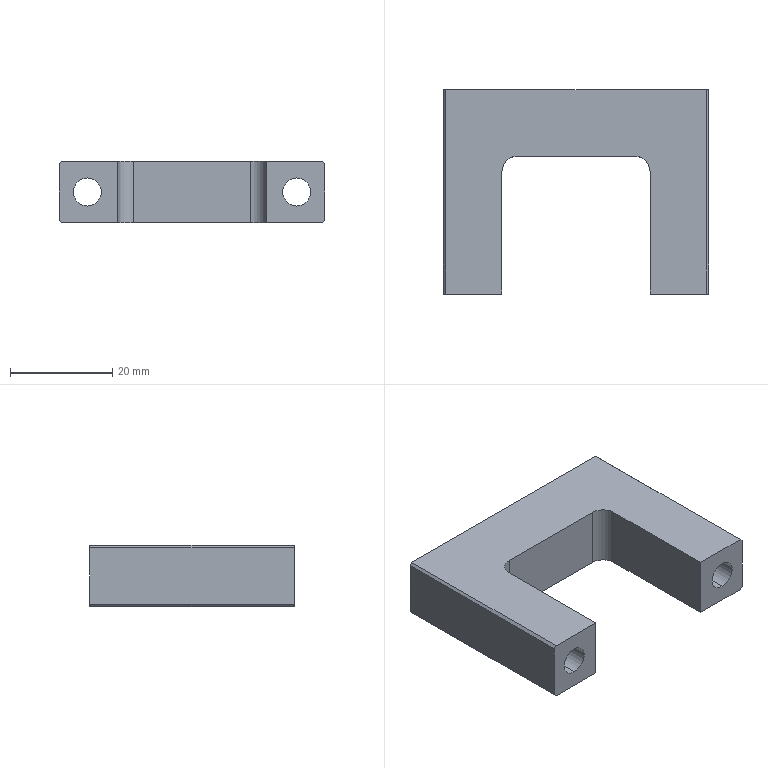Part | SolidWorks | features BaseBody 1 | 1 solid | 26 faces | box 52 x 40 x 12 mm | volume 13065 mm3 | plane 16 | cylinder 10 | commonest cylinder face diameters 5.5 x4 10 x4 6 x2
STEP:
#1=CARTESIAN_POINT('',(-20.5,-5.7,-5.));
#2=VERTEX_POINT('',#1);
#3=CARTESIAN_POINT('',(-20.5,-5.7,5.));
#4=VERTEX_POINT('',#3);
#5=CARTESIAN_POINT('',(-20.5,-5.7,0.));
#6=DIRECTION('',(0.,1.,0.));
#7=DIRECTION('',(0.,0.,1.));
#8=AXIS2_PLACEMENT_3D('',#5,#6,#7);
#9=CIRCLE('',#8,5.);
#10=EDGE_CURVE('',#2,#4,#9,.T.);
#11=ORIENTED_EDGE('',*,*,#10,.F.);
#12=CARTESIAN_POINT('',(-20.5,0.,-5.));
#13=VERTEX_POINT('',#12);
#14=CARTESIAN_POINT('',(-20.5,0.,-5.));
#15=DIRECTION('',(0.,1.,0.));
#16=VECTOR('',#15,1000.);
#17=LINE('',#14,#16);
#18=EDGE_CURVE('',#2,#13,#17,.T.);
#19=ORIENTED_EDGE('',*,*,#18,.T.);
#20=CARTESIAN_POINT('',(-20.5,0.,5.));
#21=VERTEX_POINT('',#20);
#22=CARTESIAN_POINT('',(-20.5,0.,0.));
#23=DIRECTION('',(0.,1.,0.));
#24=DIRECTION('',(0.,0.,1.));
#25=AXIS2_PLACEMENT_3D('',#22,#23,#24);
#26=CIRCLE('',#25,5.);
#27=EDGE_CURVE('',#13,#21,#26,.T.);
#28=ORIENTED_EDGE('',*,*,#27,.T.);
#29=CARTESIAN_POINT('',(-20.5,0.,5.));
#30=DIRECTION('',(0.,1.,0.));
#31=VECTOR('',#30,1000.);
#32=LINE('',#29,#31);
#33=EDGE_CURVE('',#4,#21,#32,.T.);
#34=ORIENTED_EDGE('',*,*,#33,.F.);
#35=EDGE_LOOP('',(#11,#19,#28,#34));
#36=FACE_OUTER_BOUND('',#35,.T.);
#37=CARTESIAN_POINT('',(-20.5,0.,0.));
#38=DIRECTION('',(0.,1.,0.));
#39=DIRECTION('',(0.,0.,1.));
#40=AXIS2_PLACEMENT_3D('',#37,#38,#39);
#41=CYLINDRICAL_SURFACE('',#40,5.);
#42=ADVANCED_FACE('',(#36),#41,.F.);
#43=CARTESIAN_POINT('',(-20.5,-40.,-2.75));
#44=VERTEX_POINT('',#43);
#45=CARTESIAN_POINT('',(-20.5,-40.,2.75));
#46=VERTEX_POINT('',#45);
#47=CARTESIAN_POINT('',(-20.5,-40.,0.));
#48=DIRECTION('',(0.,1.,0.));
#49=DIRECTION('',(-1.,0.,0.));
#50=AXIS2_PLACEMENT_3D('',#47,#48,#49);
#51=CIRCLE('',#50,2.75);
#52=EDGE_CURVE('',#44,#46,#51,.T.);
#53=ORIENTED_EDGE('',*,*,#52,.F.);
#54=CARTESIAN_POINT('',(-20.5,-5.7,-2.75));
#55=VERTEX_POINT('',#54);
#56=CARTESIAN_POINT('',(-20.5,0.,-2.75));
#57=DIRECTION('',(0.,1.,0.));
#58=VECTOR('',#57,1000.);
#59=LINE('',#56,#58);
#60=EDGE_CURVE('',#44,#55,#59,.T.);
#61=ORIENTED_EDGE('',*,*,#60,.T.);
#62=CARTESIAN_POINT('',(-20.5,-5.7,2.75));
#63=VERTEX_POINT('',#62);
#64=CARTESIAN_POINT('',(-20.5,-5.7,0.));
#65=DIRECTION('',(0.,1.,0.));
#66=DIRECTION('',(0.,0.,1.));
#67=AXIS2_PLACEMENT_3D('',#64,#65,#66);
#68=CIRCLE('',#67,2.75);
#69=EDGE_CURVE('',#55,#63,#68,.T.);
#70=ORIENTED_EDGE('',*,*,#69,.T.);
#71=CARTESIAN_POINT('',(-20.5,0.,2.75));
#72=DIRECTION('',(0.,1.,0.));
#73=VECTOR('',#72,1000.);
#74=LINE('',#71,#73);
#75=EDGE_CURVE('',#46,#63,#74,.T.);
#76=ORIENTED_EDGE('',*,*,#75,.F.);
#77=EDGE_LOOP('',(#53,#61,#70,#76));
#78=FACE_OUTER_BOUND('',#77,.T.);
#79=CARTESIAN_POINT('',(-20.5,0.,0.));
#80=DIRECTION('',(0.,1.,0.));
#81=DIRECTION('',(0.,0.,1.));
#82=AXIS2_PLACEMENT_3D('',#79,#80,#81);
#83=CYLINDRICAL_SURFACE('',#82,2.75);
#84=ADVANCED_FACE('',(#78),#83,.F.);
#85=CARTESIAN_POINT('',(20.5,-5.7,-5.));
#86=VERTEX_POINT('',#85);
#87=CARTESIAN_POINT('',(20.5,-5.7,5.));
#88=VERTEX_POINT('',#87);
#89=CARTESIAN_POINT('',(20.5,-5.7,0.));
#90=DIRECTION('',(0.,1.,0.));
#91=DIRECTION('',(0.,0.,1.));
#92=AXIS2_PLACEMENT_3D('',#89,#90,#91);
#93=CIRCLE('',#92,5.);
#94=EDGE_CURVE('',#86,#88,#93,.T.);
#95=ORIENTED_EDGE('',*,*,#94,.F.);
#96=CARTESIAN_POINT('',(20.5,0.,-5.));
#97=VERTEX_POINT('',#96);
#98=CARTESIAN_POINT('',(20.5,0.,-5.));
#99=DIRECTION('',(0.,1.,0.));
#100=VECTOR('',#99,1000.);
#101=LINE('',#98,#100);
#102=EDGE_CURVE('',#86,#97,#101,.T.);
#103=ORIENTED_EDGE('',*,*,#102,.T.);
#104=CARTESIAN_POINT('',(20.5,0.,5.));
#105=VERTEX_POINT('',#104);
#106=CARTESIAN_POINT('',(20.5,0.,0.));
#107=DIRECTION('',(0.,1.,0.));
#108=DIRECTION('',(0.,0.,1.));
#109=AXIS2_PLACEMENT_3D('',#106,#107,#108);
#110=CIRCLE('',#109,5.);
#111=EDGE_CURVE('',#97,#105,#110,.T.);
#112=ORIENTED_EDGE('',*,*,#111,.T.);
#113=CARTESIAN_POINT('',(20.5,0.,5.));
#114=DIRECTION('',(0.,1.,0.));
#115=VECTOR('',#114,1000.);
#116=LINE('',#113,#115);
#117=EDGE_CURVE('',#88,#105,#116,.T.);
#118=ORIENTED_EDGE('',*,*,#117,.F.);
#119=EDGE_LOOP('',(#95,#103,#112,#118));
#120=FACE_OUTER_BOUND('',#119,.T.);
#121=CARTESIAN_POINT('',(20.5,0.,0.));
#122=DIRECTION('',(0.,1.,0.));
#123=DIRECTION('',(0.,0.,1.));
#124=AXIS2_PLACEMENT_3D('',#121,#122,#123);
#125=CYLINDRICAL_SURFACE('',#124,5.);
#126=ADVANCED_FACE('',(#120),#125,.F.);
#127=CARTESIAN_POINT('',(20.5,-40.,-2.75));
#128=VERTEX_POINT('',#127);
#129=CARTESIAN_POINT('',(20.5,-40.,2.75));
#130=VERTEX_POINT('',#129);
#131=CARTESIAN_POINT('',(20.5,-40.,0.));
#132=DIRECTION('',(0.,1.,0.));
#133=DIRECTION('',(-1.,0.,0.));
#134=AXIS2_PLACEMENT_3D('',#131,#132,#133);
#135=CIRCLE('',#134,2.75);
#136=EDGE_CURVE('',#128,#130,#135,.T.);
#137=ORIENTED_EDGE('',*,*,#136,.F.);
#138=CARTESIAN_POINT('',(20.5,-5.7,-2.75));
#139=VERTEX_POINT('',#138);
#140=CARTESIAN_POINT('',(20.5,0.,-2.75));
#141=DIRECTION('',(0.,1.,0.));
#142=VECTOR('',#141,1000.);
#143=LINE('',#140,#142);
#144=EDGE_CURVE('',#128,#139,#143,.T.);
#145=ORIENTED_EDGE('',*,*,#144,.T.);
#146=CARTESIAN_POINT('',(20.5,-5.7,2.75));
#147=VERTEX_POINT('',#146);
#148=CARTESIAN_POINT('',(20.5,-5.7,0.));
#149=DIRECTION('',(0.,1.,0.));
#150=DIRECTION('',(0.,0.,1.));
#151=AXIS2_PLACEMENT_3D('',#148,#149,#150);
#152=CIRCLE('',#151,2.75);
#153=EDGE_CURVE('',#139,#147,#152,.T.);
#154=ORIENTED_EDGE('',*,*,#153,.T.);
#155=CARTESIAN_POINT('',(20.5,0.,2.75));
#156=DIRECTION('',(0.,1.,0.));
#157=VECTOR('',#156,1000.);
#158=LINE('',#155,#157);
#159=EDGE_CURVE('',#130,#147,#158,.T.);
#160=ORIENTED_EDGE('',*,*,#159,.F.);
#161=EDGE_LOOP('',(#137,#145,#154,#160));
#162=FACE_OUTER_BOUND('',#161,.T.);
#163=CARTESIAN_POINT('',(20.5,0.,0.));
#164=DIRECTION('',(0.,1.,0.));
#165=DIRECTION('',(0.,0.,1.));
#166=AXIS2_PLACEMENT_3D('',#163,#164,#165);
#167=CYLINDRICAL_SURFACE('',#166,2.75);
#168=ADVANCED_FACE('',(#162),#167,.F.);
#169=CARTESIAN_POINT('',(-14.5,-16.,6.));
#170=VERTEX_POINT('',#169);
#171=CARTESIAN_POINT('',(-11.5,-13.,6.));
#172=VERTEX_POINT('',#171);
#173=CARTESIAN_POINT('',(-11.5,-16.,6.));
#174=DIRECTION('',(0.,0.,-1.));
#175=DIRECTION('',(-1.,0.,0.));
#176=AXIS2_PLACEMENT_3D('',#173,#174,#175);
#177=CIRCLE('',#176,3.);
#178=EDGE_CURVE('',#170,#172,#177,.T.);
#179=ORIENTED_EDGE('',*,*,#178,.F.);
#180=CARTESIAN_POINT('',(-14.5,-16.,-6.));
#181=VERTEX_POINT('',#180);
#182=CARTESIAN_POINT('',(-14.5,-16.,6.));
#183=DIRECTION('',(0.,0.,1.));
#184=VECTOR('',#183,1000.);
#185=LINE('',#182,#184);
#186=EDGE_CURVE('',#181,#170,#185,.T.);
#187=ORIENTED_EDGE('',*,*,#186,.F.);
#188=CARTESIAN_POINT('',(-11.5,-13.,-6.));
#189=VERTEX_POINT('',#188);
#190=CARTESIAN_POINT('',(-11.5,-16.,-6.));
#191=DIRECTION('',(0.,0.,1.));
#192=DIRECTION('',(-1.,0.,0.));
#193=AXIS2_PLACEMENT_3D('',#190,#191,#192);
#194=CIRCLE('',#193,3.);
#195=EDGE_CURVE('',#189,#181,#194,.T.);
#196=ORIENTED_EDGE('',*,*,#195,.F.);
#197=CARTESIAN_POINT('',(-11.5,-13.,-6.));
#198=DIRECTION('',(0.,0.,-1.));
#199=VECTOR('',#198,1000.);
#200=LINE('',#197,#199);
#201=EDGE_CURVE('',#172,#189,#200,.T.);
#202=ORIENTED_EDGE('',*,*,#201,.F.);
#203=EDGE_LOOP('',(#179,#187,#196,#202));
#204=FACE_OUTER_BOUND('',#203,.T.);
#205=CARTESIAN_POINT('',(-11.5,-16.,6.));
#206=DIRECTION('',(0.,0.,1.));
#207=DIRECTION('',(1.,0.,0.));
#208=AXIS2_PLACEMENT_3D('',#205,#206,#207);
#209=CYLINDRICAL_SURFACE('',#208,3.);
#210=ADVANCED_FACE('',(#204),#209,.F.);
#211=CARTESIAN_POINT('',(11.5,-13.,6.));
#212=VERTEX_POINT('',#211);
#213=CARTESIAN_POINT('',(14.5,-16.,6.));
#214=VERTEX_POINT('',#213);
#215=CARTESIAN_POINT('',(11.5,-16.,6.));
#216=DIRECTION('',(0.,0.,-1.));
#217=DIRECTION('',(-1.,0.,0.));
#218=AXIS2_PLACEMENT_3D('',#215,#216,#217);
#219=CIRCLE('',#218,3.);
#220=EDGE_CURVE('',#212,#214,#219,.T.);
#221=ORIENTED_EDGE('',*,*,#220,.F.);
#222=CARTESIAN_POINT('',(11.5,-13.,-6.));
#223=VERTEX_POINT('',#222);
#224=CARTESIAN_POINT('',(11.5,-13.,6.));
#225=DIRECTION('',(0.,0.,1.));
#226=VECTOR('',#225,1000.);
#227=LINE('',#224,#226);
#228=EDGE_CURVE('',#223,#212,#227,.T.);
#229=ORIENTED_EDGE('',*,*,#228,.F.);
#230=CARTESIAN_POINT('',(14.5,-16.,-6.));
#231=VERTEX_POINT('',#230);
#232=CARTESIAN_POINT('',(11.5,-16.,-6.));
#233=DIRECTION('',(0.,0.,1.));
#234=DIRECTION('',(-1.,0.,0.));
#235=AXIS2_PLACEMENT_3D('',#232,#233,#234);
#236=CIRCLE('',#235,3.);
#237=EDGE_CURVE('',#231,#223,#236,.T.);
#238=ORIENTED_EDGE('',*,*,#237,.F.);
#239=CARTESIAN_POINT('',(14.5,-16.,-6.));
#240=DIRECTION('',(0.,0.,-1.));
#241=VECTOR('',#240,1000.);
#242=LINE('',#239,#241);
#243=EDGE_CURVE('',#214,#231,#242,.T.);
#244=ORIENTED_EDGE('',*,*,#243,.F.);
#245=EDGE_LOOP('',(#221,#229,#238,#244));
#246=FACE_OUTER_BOUND('',#245,.T.);
#247=CARTESIAN_POINT('',(11.5,-16.,6.));
#248=DIRECTION('',(0.,0.,1.));
#249=DIRECTION('',(1.,0.,0.));
#250=AXIS2_PLACEMENT_3D('',#247,#248,#249);
#251=CYLINDRICAL_SURFACE('',#250,3.);
#252=ADVANCED_FACE('',(#246),#251,.F.);
#253=CARTESIAN_POINT('',(-26.,0.,5.5));
#254=VERTEX_POINT('',#253);
#255=CARTESIAN_POINT('',(-25.5,0.,6.));
#256=VERTEX_POINT('',#255);
#257=CARTESIAN_POINT('',(-25.5,0.,6.));
#258=DIRECTION('',(0.7071,0.,0.7071));
#259=VECTOR('',#258,1000.);
#260=LINE('',#257,#259);
#261=EDGE_CURVE('',#254,#256,#260,.T.);
#262=ORIENTED_EDGE('',*,*,#261,.F.);
#263=CARTESIAN_POINT('',(-26.,-40.,5.5));
#264=VERTEX_POINT('',#263);
#265=CARTESIAN_POINT('',(-26.,-40.,5.5));
#266=DIRECTION('',(0.,1.,0.));
#267=VECTOR('',#266,1000.);
#268=LINE('',#265,#267);
#269=EDGE_CURVE('',#264,#254,#268,.T.);
#270=ORIENTED_EDGE('',*,*,#269,.F.);
#271=CARTESIAN_POINT('',(-25.5,-40.,6.));
#272=VERTEX_POINT('',#271);
#273=CARTESIAN_POINT('',(-25.5,-40.,6.));
#274=DIRECTION('',(-0.7071,0.,-0.7071));
#275=VECTOR('',#274,1000.);
#276=LINE('',#273,#275);
#277=EDGE_CURVE('',#272,#264,#276,.T.);
#278=ORIENTED_EDGE('',*,*,#277,.F.);
#279=CARTESIAN_POINT('',(-25.5,0.,6.));
#280=DIRECTION('',(0.,-1.,0.));
#281=VECTOR('',#280,1000.);
#282=LINE('',#279,#281);
#283=EDGE_CURVE('',#256,#272,#282,.T.);
#284=ORIENTED_EDGE('',*,*,#283,.F.);
#285=EDGE_LOOP('',(#262,#270,#278,#284));
#286=FACE_OUTER_BOUND('',#285,.T.);
#287=CARTESIAN_POINT('',(-25.5,0.,6.));
#288=DIRECTION('',(0.7071,0.,-0.7071));
#289=DIRECTION('',(0.,-1.,0.));
#290=AXIS2_PLACEMENT_3D('',#287,#288,#289);
#291=PLANE('',#290);
#292=ADVANCED_FACE('',(#286),#291,.F.);
#293=CARTESIAN_POINT('',(-25.5,0.,-6.));
#294=VERTEX_POINT('',#293);
#295=CARTESIAN_POINT('',(-26.,0.,-5.5));
#296=VERTEX_POINT('',#295);
#297=CARTESIAN_POINT('',(-26.,0.,-5.5));
#298=DIRECTION('',(-0.7071,0.,0.7071));
#299=VECTOR('',#298,1000.);
#300=LINE('',#297,#299);
#301=EDGE_CURVE('',#294,#296,#300,.T.);
#302=ORIENTED_EDGE('',*,*,#301,.F.);
#303=CARTESIAN_POINT('',(-25.5,-40.,-6.));
#304=VERTEX_POINT('',#303);
#305=CARTESIAN_POINT('',(-25.5,0.,-6.));
#306=DIRECTION('',(0.,1.,0.));
#307=VECTOR('',#306,1000.);
#308=LINE('',#305,#307);
#309=EDGE_CURVE('',#304,#294,#308,.T.);
#310=ORIENTED_EDGE('',*,*,#309,.F.);
#311=CARTESIAN_POINT('',(-26.,-40.,-5.5));
#312=VERTEX_POINT('',#311);
#313=CARTESIAN_POINT('',(-26.,-40.,-5.5));
#314=DIRECTION('',(0.7071,0.,-0.7071));
#315=VECTOR('',#314,1000.);
#316=LINE('',#313,#315);
#317=EDGE_CURVE('',#312,#304,#316,.T.);
#318=ORIENTED_EDGE('',*,*,#317,.F.);
#319=CARTESIAN_POINT('',(-26.,-40.,-5.5));
#320=DIRECTION('',(0.,-1.,0.));
#321=VECTOR('',#320,1000.);
#322=LINE('',#319,#321);
#323=EDGE_CURVE('',#296,#312,#322,.T.);
#324=ORIENTED_EDGE('',*,*,#323,.F.);
#325=EDGE_LOOP('',(#302,#310,#318,#324));
#326=FACE_OUTER_BOUND('',#325,.T.);
#327=CARTESIAN_POINT('',(-26.,-40.,-5.5));
#328=DIRECTION('',(-0.7071,0.,-0.7071));
#329=DIRECTION('',(-0.7071,0.,0.7071));
#330=AXIS2_PLACEMENT_3D('',#327,#328,#329);
#331=PLANE('',#330);
#332=ADVANCED_FACE('',(#326),#331,.T.);
#333=CARTESIAN_POINT('',(26.,-40.,5.5));
#334=VERTEX_POINT('',#333);
#335=CARTESIAN_POINT('',(25.5,-40.,6.));
#336=VERTEX_POINT('',#335);
#337=CARTESIAN_POINT('',(25.5,-40.,6.));
#338=DIRECTION('',(-0.7071,0.,0.7071));
#339=VECTOR('',#338,1000.);
#340=LINE('',#337,#339);
#341=EDGE_CURVE('',#334,#336,#340,.T.);
#342=ORIENTED_EDGE('',*,*,#341,.F.);
#343=CARTESIAN_POINT('',(26.,0.,5.5));
#344=VERTEX_POINT('',#343);
#345=CARTESIAN_POINT('',(26.,0.,5.5));
#346=DIRECTION('',(0.,-1.,0.));
#347=VECTOR('',#346,1000.);
#348=LINE('',#345,#347);
#349=EDGE_CURVE('',#344,#334,#348,.T.);
#350=ORIENTED_EDGE('',*,*,#349,.F.);
#351=CARTESIAN_POINT('',(25.5,0.,6.));
#352=VERTEX_POINT('',#351);
#353=CARTESIAN_POINT('',(25.5,0.,6.));
#354=DIRECTION('',(0.7071,0.,-0.7071));
#355=VECTOR('',#354,1000.);
#356=LINE('',#353,#355);
#357=EDGE_CURVE('',#352,#344,#356,.T.);
#358=ORIENTED_EDGE('',*,*,#357,.F.);
#359=CARTESIAN_POINT('',(25.5,0.,6.));
#360=DIRECTION('',(0.,1.,0.));
#361=VECTOR('',#360,1000.);
#362=LINE('',#359,#361);
#363=EDGE_CURVE('',#336,#352,#362,.T.);
#364=ORIENTED_EDGE('',*,*,#363,.F.);
#365=EDGE_LOOP('',(#342,#350,#358,#364));
#366=FACE_OUTER_BOUND('',#365,.T.);
#367=CARTESIAN_POINT('',(25.5,0.,6.));
#368=DIRECTION('',(-0.7071,0.,-0.7071));
#369=DIRECTION('',(-0.7071,0.,0.7071));
#370=AXIS2_PLACEMENT_3D('',#367,#368,#369);
#371=PLANE('',#370);
#372=ADVANCED_FACE('',(#366),#371,.F.);
#373=CARTESIAN_POINT('',(25.5,-40.,-6.));
#374=VERTEX_POINT('',#373);
#375=CARTESIAN_POINT('',(26.,-40.,-5.5));
#376=VERTEX_POINT('',#375);
#377=CARTESIAN_POINT('',(26.,-40.,-5.5));
#378=DIRECTION('',(0.7071,0.,0.7071));
#379=VECTOR('',#378,1000.);
#380=LINE('',#377,#379);
#381=EDGE_CURVE('',#374,#376,#380,.T.);
#382=ORIENTED_EDGE('',*,*,#381,.F.);
#383=CARTESIAN_POINT('',(25.5,0.,-6.));
#384=VERTEX_POINT('',#383);
#385=CARTESIAN_POINT('',(25.5,-40.,-6.));
#386=DIRECTION('',(0.,-1.,0.));
#387=VECTOR('',#386,1000.);
#388=LINE('',#385,#387);
#389=EDGE_CURVE('',#384,#374,#388,.T.);
#390=ORIENTED_EDGE('',*,*,#389,.F.);
#391=CARTESIAN_POINT('',(26.,0.,-5.5));
#392=VERTEX_POINT('',#391);
#393=CARTESIAN_POINT('',(26.,0.,-5.5));
#394=DIRECTION('',(-0.7071,0.,-0.7071));
#395=VECTOR('',#394,1000.);
#396=LINE('',#393,#395);
#397=EDGE_CURVE('',#392,#384,#396,.T.);
#398=ORIENTED_EDGE('',*,*,#397,.F.);
#399=CARTESIAN_POINT('',(26.,0.,-5.5));
#400=DIRECTION('',(0.,1.,0.));
#401=VECTOR('',#400,1000.);
#402=LINE('',#399,#401);
#403=EDGE_CURVE('',#376,#392,#402,.T.);
#404=ORIENTED_EDGE('',*,*,#403,.F.);
#405=EDGE_LOOP('',(#382,#390,#398,#404));
#406=FACE_OUTER_BOUND('',#405,.T.);
#407=CARTESIAN_POINT('',(26.,0.,-5.5));
#408=DIRECTION('',(0.7071,0.,-0.7071));
#409=DIRECTION('',(0.,-1.,0.));
#410=AXIS2_PLACEMENT_3D('',#407,#408,#409);
#411=PLANE('',#410);
#412=ADVANCED_FACE('',(#406),#411,.T.);
#413=CARTESIAN_POINT('',(-20.5,-5.7,0.));
#414=DIRECTION('',(0.,1.,0.));
#415=DIRECTION('',(0.,0.,1.));
#416=AXIS2_PLACEMENT_3D('',#413,#414,#415);
#417=CIRCLE('',#416,2.75);
#418=EDGE_CURVE('',#63,#55,#417,.T.);
#419=ORIENTED_EDGE('',*,*,#418,.F.);
#420=ORIENTED_EDGE('',*,*,#69,.F.);
#421=EDGE_LOOP('',(#419,#420));
#422=FACE_BOUND('',#421,.T.);
#423=CARTESIAN_POINT('',(-20.5,-5.7,0.));
#424=DIRECTION('',(0.,1.,0.));
#425=DIRECTION('',(0.,0.,1.));
#426=AXIS2_PLACEMENT_3D('',#423,#424,#425);
#427=CIRCLE('',#426,5.);
#428=EDGE_CURVE('',#4,#2,#427,.T.);
#429=ORIENTED_EDGE('',*,*,#428,.T.);
#430=ORIENTED_EDGE('',*,*,#10,.T.);
#431=EDGE_LOOP('',(#429,#430));
#432=FACE_OUTER_BOUND('',#431,.T.);
#433=CARTESIAN_POINT('',(-17.75,-5.7,0.));
#434=DIRECTION('',(0.,-1.,0.));
#435=DIRECTION('',(0.,0.,-1.));
#436=AXIS2_PLACEMENT_3D('',#433,#434,#435);
#437=PLANE('',#436);
#438=ADVANCED_FACE('',(#422,#432),#437,.F.);
#439=CARTESIAN_POINT('',(20.5,-5.7,0.));
#440=DIRECTION('',(0.,1.,0.));
#441=DIRECTION('',(0.,0.,1.));
#442=AXIS2_PLACEMENT_3D('',#439,#440,#441);
#443=CIRCLE('',#442,2.75);
#444=EDGE_CURVE('',#147,#139,#443,.T.);
#445=ORIENTED_EDGE('',*,*,#444,.F.);
#446=ORIENTED_EDGE('',*,*,#153,.F.);
#447=EDGE_LOOP('',(#445,#446));
#448=FACE_BOUND('',#447,.T.);
#449=CARTESIAN_POINT('',(20.5,-5.7,0.));
#450=DIRECTION('',(0.,1.,0.));
#451=DIRECTION('',(0.,0.,1.));
#452=AXIS2_PLACEMENT_3D('',#449,#450,#451);
#453=CIRCLE('',#452,5.);
#454=EDGE_CURVE('',#88,#86,#453,.T.);
#455=ORIENTED_EDGE('',*,*,#454,.T.);
#456=ORIENTED_EDGE('',*,*,#94,.T.);
#457=EDGE_LOOP('',(#455,#456));
#458=FACE_OUTER_BOUND('',#457,.T.);
#459=CARTESIAN_POINT('',(23.25,-5.7,0.));
#460=DIRECTION('',(0.,-1.,0.));
#461=DIRECTION('',(0.,0.,-1.));
#462=AXIS2_PLACEMENT_3D('',#459,#460,#461);
#463=PLANE('',#462);
#464=ADVANCED_FACE('',(#448,#458),#463,.F.);
#465=CARTESIAN_POINT('',(-26.,0.,-6.));
#466=DIRECTION('',(-1.,0.,0.));
#467=VECTOR('',#466,1000.);
#468=LINE('',#465,#467);
#469=EDGE_CURVE('',#384,#294,#468,.T.);
#470=ORIENTED_EDGE('',*,*,#469,.F.);
#471=ORIENTED_EDGE('',*,*,#389,.T.);
#472=CARTESIAN_POINT('',(14.5,-40.,-6.));
#473=VERTEX_POINT('',#472);
#474=CARTESIAN_POINT('',(26.,-40.,-6.));
#475=DIRECTION('',(1.,0.,0.));
#476=VECTOR('',#475,1000.);
#477=LINE('',#474,#476);
#478=EDGE_CURVE('',#473,#374,#477,.T.);
#479=ORIENTED_EDGE('',*,*,#478,.F.);
#480=CARTESIAN_POINT('',(14.5,-40.,-6.));
#481=DIRECTION('',(0.,-1.,0.));
#482=VECTOR('',#481,1000.);
#483=LINE('',#480,#482);
#484=EDGE_CURVE('',#231,#473,#483,.T.);
#485=ORIENTED_EDGE('',*,*,#484,.F.);
#486=ORIENTED_EDGE('',*,*,#237,.T.);
#487=CARTESIAN_POINT('',(14.5,-13.,-6.));
#488=DIRECTION('',(1.,0.,0.));
#489=VECTOR('',#488,1000.);
#490=LINE('',#487,#489);
#491=EDGE_CURVE('',#189,#223,#490,.T.);
#492=ORIENTED_EDGE('',*,*,#491,.F.);
#493=ORIENTED_EDGE('',*,*,#195,.T.);
#494=CARTESIAN_POINT('',(-14.5,-40.,-6.));
#495=VERTEX_POINT('',#494);
#496=CARTESIAN_POINT('',(-14.5,-13.,-6.));
#497=DIRECTION('',(0.,1.,0.));
#498=VECTOR('',#497,1000.);
#499=LINE('',#496,#498);
#500=EDGE_CURVE('',#495,#181,#499,.T.);
#501=ORIENTED_EDGE('',*,*,#500,.F.);
#502=CARTESIAN_POINT('',(-14.5,-40.,-6.));
#503=DIRECTION('',(1.,0.,0.));
#504=VECTOR('',#503,1000.);
#505=LINE('',#502,#504);
#506=EDGE_CURVE('',#304,#495,#505,.T.);
#507=ORIENTED_EDGE('',*,*,#506,.F.);
#508=ORIENTED_EDGE('',*,*,#309,.T.);
#509=EDGE_LOOP('',(#470,#471,#479,#485,#486,#492,#493,#501,#507,#508));
#510=FACE_OUTER_BOUND('',#509,.T.);
#511=CARTESIAN_POINT('',(0.,0.,-6.));
#512=DIRECTION('',(0.,0.,-1.));
#513=DIRECTION('',(0.,-1.,0.));
#514=AXIS2_PLACEMENT_3D('',#511,#512,#513);
#515=PLANE('',#514);
#516=ADVANCED_FACE('',(#510),#515,.T.);
#517=CARTESIAN_POINT('',(14.5,-40.,6.));
#518=VERTEX_POINT('',#517);
#519=CARTESIAN_POINT('',(26.,-40.,6.));
#520=DIRECTION('',(1.,0.,0.));
#521=VECTOR('',#520,1000.);
#522=LINE('',#519,#521);
#523=EDGE_CURVE('',#518,#336,#522,.T.);
#524=ORIENTED_EDGE('',*,*,#523,.T.);
#525=ORIENTED_EDGE('',*,*,#363,.T.);
#526=CARTESIAN_POINT('',(-26.,0.,6.));
#527=DIRECTION('',(-1.,0.,0.));
#528=VECTOR('',#527,1000.);
#529=LINE('',#526,#528);
#530=EDGE_CURVE('',#352,#256,#529,.T.);
#531=ORIENTED_EDGE('',*,*,#530,.T.);
#532=ORIENTED_EDGE('',*,*,#283,.T.);
#533=CARTESIAN_POINT('',(-14.5,-40.,6.));
#534=VERTEX_POINT('',#533);
#535=CARTESIAN_POINT('',(-14.5,-40.,6.));
#536=DIRECTION('',(1.,0.,0.));
#537=VECTOR('',#536,1000.);
#538=LINE('',#535,#537);
#539=EDGE_CURVE('',#272,#534,#538,.T.);
#540=ORIENTED_EDGE('',*,*,#539,.T.);
#541=CARTESIAN_POINT('',(-14.5,-13.,6.));
#542=DIRECTION('',(0.,1.,0.));
#543=VECTOR('',#542,1000.);
#544=LINE('',#541,#543);
#545=EDGE_CURVE('',#534,#170,#544,.T.);
#546=ORIENTED_EDGE('',*,*,#545,.T.);
#547=ORIENTED_EDGE('',*,*,#178,.T.);
#548=CARTESIAN_POINT('',(14.5,-13.,6.));
#549=DIRECTION('',(1.,0.,0.));
#550=VECTOR('',#549,1000.);
#551=LINE('',#548,#550);
#552=EDGE_CURVE('',#172,#212,#551,.T.);
#553=ORIENTED_EDGE('',*,*,#552,.T.);
#554=ORIENTED_EDGE('',*,*,#220,.T.);
#555=CARTESIAN_POINT('',(14.5,-40.,6.));
#556=DIRECTION('',(0.,-1.,0.));
#557=VECTOR('',#556,1000.);
#558=LINE('',#555,#557);
#559=EDGE_CURVE('',#214,#518,#558,.T.);
#560=ORIENTED_EDGE('',*,*,#559,.T.);
#561=EDGE_LOOP('',(#524,#525,#531,#532,#540,#546,#547,#553,#554,#560));
#562=FACE_OUTER_BOUND('',#561,.T.);
#563=CARTESIAN_POINT('',(0.,0.,6.));
#564=DIRECTION('',(0.,0.,-1.));
#565=DIRECTION('',(0.,-1.,0.));
#566=AXIS2_PLACEMENT_3D('',#563,#564,#565);
#567=PLANE('',#566);
#568=ADVANCED_FACE('',(#562),#567,.F.);
#569=CARTESIAN_POINT('',(-26.,0.,6.));
#570=DIRECTION('',(0.,0.,-1.));
#571=VECTOR('',#570,1000.);
#572=LINE('',#569,#571);
#573=EDGE_CURVE('',#254,#296,#572,.T.);
#574=ORIENTED_EDGE('',*,*,#573,.T.);
#575=ORIENTED_EDGE('',*,*,#323,.T.);
#576=CARTESIAN_POINT('',(-26.,-40.,6.));
#577=DIRECTION('',(0.,0.,-1.));
#578=VECTOR('',#577,1000.);
#579=LINE('',#576,#578);
#580=EDGE_CURVE('',#264,#312,#579,.T.);
#581=ORIENTED_EDGE('',*,*,#580,.F.);
#582=ORIENTED_EDGE('',*,*,#269,.T.);
#583=EDGE_LOOP('',(#574,#575,#581,#582));
#584=FACE_OUTER_BOUND('',#583,.T.);
#585=CARTESIAN_POINT('',(-26.,-40.,6.));
#586=DIRECTION('',(1.,0.,0.));
#587=DIRECTION('',(0.,-1.,0.));
#588=AXIS2_PLACEMENT_3D('',#585,#586,#587);
#589=PLANE('',#588);
#590=ADVANCED_FACE('',(#584),#589,.F.);
#591=CARTESIAN_POINT('',(26.,-40.,6.));
#592=DIRECTION('',(0.,0.,-1.));
#593=VECTOR('',#592,1000.);
#594=LINE('',#591,#593);
#595=EDGE_CURVE('',#334,#376,#594,.T.);
#596=ORIENTED_EDGE('',*,*,#595,.T.);
#597=ORIENTED_EDGE('',*,*,#403,.T.);
#598=CARTESIAN_POINT('',(26.,0.,6.));
#599=DIRECTION('',(0.,0.,-1.));
#600=VECTOR('',#599,1000.);
#601=LINE('',#598,#600);
#602=EDGE_CURVE('',#344,#392,#601,.T.);
#603=ORIENTED_EDGE('',*,*,#602,.F.);
#604=ORIENTED_EDGE('',*,*,#349,.T.);
#605=EDGE_LOOP('',(#596,#597,#603,#604));
#606=FACE_OUTER_BOUND('',#605,.T.);
#607=CARTESIAN_POINT('',(26.,0.,6.));
#608=DIRECTION('',(-1.,0.,0.));
#609=DIRECTION('',(0.,1.,0.));
#610=AXIS2_PLACEMENT_3D('',#607,#608,#609);
#611=PLANE('',#610);
#612=ADVANCED_FACE('',(#606),#611,.F.);
#613=CARTESIAN_POINT('',(20.5,-40.,0.));
#614=DIRECTION('',(0.,1.,0.));
#615=DIRECTION('',(-1.,0.,0.));
#616=AXIS2_PLACEMENT_3D('',#613,#614,#615);
#617=CIRCLE('',#616,2.75);
#618=EDGE_CURVE('',#130,#128,#617,.T.);
#619=ORIENTED_EDGE('',*,*,#618,.T.);
#620=ORIENTED_EDGE('',*,*,#136,.T.);
#621=EDGE_LOOP('',(#619,#620));
#622=FACE_BOUND('',#621,.T.);
#623=ORIENTED_EDGE('',*,*,#478,.T.);
#624=ORIENTED_EDGE('',*,*,#381,.T.);
#625=ORIENTED_EDGE('',*,*,#595,.F.);
#626=ORIENTED_EDGE('',*,*,#341,.T.);
#627=ORIENTED_EDGE('',*,*,#523,.F.);
#628=CARTESIAN_POINT('',(14.5,-40.,6.));
#629=DIRECTION('',(0.,0.,-1.));
#630=VECTOR('',#629,1000.);
#631=LINE('',#628,#630);
#632=EDGE_CURVE('',#518,#473,#631,.T.);
#633=ORIENTED_EDGE('',*,*,#632,.T.);
#634=EDGE_LOOP('',(#623,#624,#625,#626,#627,#633));
#635=FACE_OUTER_BOUND('',#634,.T.);
#636=CARTESIAN_POINT('',(26.,-40.,6.));
#637=DIRECTION('',(0.,1.,0.));
#638=DIRECTION('',(1.,0.,0.));
#639=AXIS2_PLACEMENT_3D('',#636,#637,#638);
#640=PLANE('',#639);
#641=ADVANCED_FACE('',(#622,#635),#640,.F.);
#642=ORIENTED_EDGE('',*,*,#559,.F.);
#643=ORIENTED_EDGE('',*,*,#243,.T.);
#644=ORIENTED_EDGE('',*,*,#484,.T.);
#645=ORIENTED_EDGE('',*,*,#632,.F.);
#646=EDGE_LOOP('',(#642,#643,#644,#645));
#647=FACE_OUTER_BOUND('',#646,.T.);
#648=CARTESIAN_POINT('',(14.5,-40.,6.));
#649=DIRECTION('',(1.,0.,0.));
#650=DIRECTION('',(0.,1.,0.));
#651=AXIS2_PLACEMENT_3D('',#648,#649,#650);
#652=PLANE('',#651);
#653=ADVANCED_FACE('',(#647),#652,.F.);
#654=ORIENTED_EDGE('',*,*,#491,.T.);
#655=ORIENTED_EDGE('',*,*,#228,.T.);
#656=ORIENTED_EDGE('',*,*,#552,.F.);
#657=ORIENTED_EDGE('',*,*,#201,.T.);
#658=EDGE_LOOP('',(#654,#655,#656,#657));
#659=FACE_OUTER_BOUND('',#658,.T.);
#660=CARTESIAN_POINT('',(14.5,-13.,6.));
#661=DIRECTION('',(0.,1.,0.));
#662=DIRECTION('',(1.,0.,0.));
#663=AXIS2_PLACEMENT_3D('',#660,#661,#662);
#664=PLANE('',#663);
#665=ADVANCED_FACE('',(#659),#664,.F.);
#666=ORIENTED_EDGE('',*,*,#500,.T.);
#667=ORIENTED_EDGE('',*,*,#186,.T.);
#668=ORIENTED_EDGE('',*,*,#545,.F.);
#669=CARTESIAN_POINT('',(-14.5,-40.,6.));
#670=DIRECTION('',(0.,0.,-1.));
#671=VECTOR('',#670,1000.);
#672=LINE('',#669,#671);
#673=EDGE_CURVE('',#534,#495,#672,.T.);
#674=ORIENTED_EDGE('',*,*,#673,.T.);
#675=EDGE_LOOP('',(#666,#667,#668,#674));
#676=FACE_OUTER_BOUND('',#675,.T.);
#677=CARTESIAN_POINT('',(-14.5,-13.,6.));
#678=DIRECTION('',(-1.,0.,0.));
#679=DIRECTION('',(0.,0.,1.));
#680=AXIS2_PLACEMENT_3D('',#677,#678,#679);
#681=PLANE('',#680);
#682=ADVANCED_FACE('',(#676),#681,.F.);
#683=CARTESIAN_POINT('',(-20.5,-40.,0.));
#684=DIRECTION('',(0.,1.,0.));
#685=DIRECTION('',(-1.,0.,0.));
#686=AXIS2_PLACEMENT_3D('',#683,#684,#685);
#687=CIRCLE('',#686,2.75);
#688=EDGE_CURVE('',#46,#44,#687,.T.);
#689=ORIENTED_EDGE('',*,*,#688,.T.);
#690=ORIENTED_EDGE('',*,*,#52,.T.);
#691=EDGE_LOOP('',(#689,#690));
#692=FACE_BOUND('',#691,.T.);
#693=ORIENTED_EDGE('',*,*,#580,.T.);
#694=ORIENTED_EDGE('',*,*,#317,.T.);
#695=ORIENTED_EDGE('',*,*,#506,.T.);
#696=ORIENTED_EDGE('',*,*,#673,.F.);
#697=ORIENTED_EDGE('',*,*,#539,.F.);
#698=ORIENTED_EDGE('',*,*,#277,.T.);
#699=EDGE_LOOP('',(#693,#694,#695,#696,#697,#698));
#700=FACE_OUTER_BOUND('',#699,.T.);
#701=CARTESIAN_POINT('',(-14.5,-40.,6.));
#702=DIRECTION('',(0.,1.,0.));
#703=DIRECTION('',(1.,0.,0.));
#704=AXIS2_PLACEMENT_3D('',#701,#702,#703);
#705=PLANE('',#704);
#706=ADVANCED_FACE('',(#692,#700),#705,.F.);
#707=CARTESIAN_POINT('',(20.5,0.,0.));
#708=DIRECTION('',(0.,1.,0.));
#709=DIRECTION('',(0.,0.,1.));
#710=AXIS2_PLACEMENT_3D('',#707,#708,#709);
#711=CIRCLE('',#710,5.);
#712=EDGE_CURVE('',#105,#97,#711,.T.);
#713=ORIENTED_EDGE('',*,*,#712,.F.);
#714=ORIENTED_EDGE('',*,*,#111,.F.);
#715=EDGE_LOOP('',(#713,#714));
#716=FACE_BOUND('',#715,.T.);
#717=CARTESIAN_POINT('',(-20.5,0.,0.));
#718=DIRECTION('',(0.,1.,0.));
#719=DIRECTION('',(0.,0.,1.));
#720=AXIS2_PLACEMENT_3D('',#717,#718,#719);
#721=CIRCLE('',#720,5.);
#722=EDGE_CURVE('',#21,#13,#721,.T.);
#723=ORIENTED_EDGE('',*,*,#722,.F.);
#724=ORIENTED_EDGE('',*,*,#27,.F.);
#725=EDGE_LOOP('',(#723,#724));
#726=FACE_BOUND('',#725,.T.);
#727=ORIENTED_EDGE('',*,*,#602,.T.);
#728=ORIENTED_EDGE('',*,*,#397,.T.);
#729=ORIENTED_EDGE('',*,*,#469,.T.);
#730=ORIENTED_EDGE('',*,*,#301,.T.);
#731=ORIENTED_EDGE('',*,*,#573,.F.);
#732=ORIENTED_EDGE('',*,*,#261,.T.);
#733=ORIENTED_EDGE('',*,*,#530,.F.);
#734=ORIENTED_EDGE('',*,*,#357,.T.);
#735=EDGE_LOOP('',(#727,#728,#729,#730,#731,#732,#733,#734));
#736=FACE_OUTER_BOUND('',#735,.T.);
#737=CARTESIAN_POINT('',(-26.,0.,6.));
#738=DIRECTION('',(0.,-1.,0.));
#739=DIRECTION('',(0.,0.,-1.));
#740=AXIS2_PLACEMENT_3D('',#737,#738,#739);
#741=PLANE('',#740);
#742=ADVANCED_FACE('',(#716,#726,#736),#741,.F.);
#743=ORIENTED_EDGE('',*,*,#144,.F.);
#744=ORIENTED_EDGE('',*,*,#618,.F.);
#745=ORIENTED_EDGE('',*,*,#159,.T.);
#746=ORIENTED_EDGE('',*,*,#444,.T.);
#747=EDGE_LOOP('',(#743,#744,#745,#746));
#748=FACE_OUTER_BOUND('',#747,.T.);
#749=CARTESIAN_POINT('',(20.5,0.,0.));
#750=DIRECTION('',(0.,1.,0.));
#751=DIRECTION('',(0.,0.,1.));
#752=AXIS2_PLACEMENT_3D('',#749,#750,#751);
#753=CYLINDRICAL_SURFACE('',#752,2.75);
#754=ADVANCED_FACE('',(#748),#753,.F.);
#755=ORIENTED_EDGE('',*,*,#102,.F.);
#756=ORIENTED_EDGE('',*,*,#454,.F.);
#757=ORIENTED_EDGE('',*,*,#117,.T.);
#758=ORIENTED_EDGE('',*,*,#712,.T.);
#759=EDGE_LOOP('',(#755,#756,#757,#758));
#760=FACE_OUTER_BOUND('',#759,.T.);
#761=CARTESIAN_POINT('',(20.5,0.,0.));
#762=DIRECTION('',(0.,1.,0.));
#763=DIRECTION('',(0.,0.,1.));
#764=AXIS2_PLACEMENT_3D('',#761,#762,#763);
#765=CYLINDRICAL_SURFACE('',#764,5.);
#766=ADVANCED_FACE('',(#760),#765,.F.);
#767=ORIENTED_EDGE('',*,*,#60,.F.);
#768=ORIENTED_EDGE('',*,*,#688,.F.);
#769=ORIENTED_EDGE('',*,*,#75,.T.);
#770=ORIENTED_EDGE('',*,*,#418,.T.);
#771=EDGE_LOOP('',(#767,#768,#769,#770));
#772=FACE_OUTER_BOUND('',#771,.T.);
#773=CARTESIAN_POINT('',(-20.5,0.,0.));
#774=DIRECTION('',(0.,1.,0.));
#775=DIRECTION('',(0.,0.,1.));
#776=AXIS2_PLACEMENT_3D('',#773,#774,#775);
#777=CYLINDRICAL_SURFACE('',#776,2.75);
#778=ADVANCED_FACE('',(#772),#777,.F.);
#779=ORIENTED_EDGE('',*,*,#18,.F.);
#780=ORIENTED_EDGE('',*,*,#428,.F.);
#781=ORIENTED_EDGE('',*,*,#33,.T.);
#782=ORIENTED_EDGE('',*,*,#722,.T.);
#783=EDGE_LOOP('',(#779,#780,#781,#782));
#784=FACE_OUTER_BOUND('',#783,.T.);
#785=CARTESIAN_POINT('',(-20.5,0.,0.));
#786=DIRECTION('',(0.,1.,0.));
#787=DIRECTION('',(0.,0.,1.));
#788=AXIS2_PLACEMENT_3D('',#785,#786,#787);
#789=CYLINDRICAL_SURFACE('',#788,5.);
#790=ADVANCED_FACE('',(#784),#789,.F.);
#791=CLOSED_SHELL('',(#42,#84,#126,#168,#210,#252,#292,#332,#372,#412,#438,#464,#516,#568,#590,#612,#641,#653,#665,#682,#706,#742,#754,#766,#778,#790));
#792=MANIFOLD_SOLID_BREP('',#791);
#793=CARTESIAN_POINT('',(0.,0.,0.));
#794=DIRECTION('',(0.,0.,1.));
#795=DIRECTION('',(1.,0.,0.));
#796=AXIS2_PLACEMENT_3D('',#793,#794,#795);
#797=(LENGTH_UNIT()NAMED_UNIT(*)SI_UNIT(.MILLI.,.METRE.));
#798=UNCERTAINTY_MEASURE_WITH_UNIT(LENGTH_MEASURE(0.00001),#797,'','');
#799=(NAMED_UNIT(*)PLANE_ANGLE_UNIT()SI_UNIT($,.RADIAN.));
#800=(NAMED_UNIT(*)SI_UNIT($,.STERADIAN.)SOLID_ANGLE_UNIT());
#801=(GEOMETRIC_REPRESENTATION_CONTEXT(3)GLOBAL_UNCERTAINTY_ASSIGNED_CONTEXT((#798))GLOBAL_UNIT_ASSIGNED_CONTEXT((#797,#799,#800))REPRESENTATION_CONTEXT('',''));
#802=ADVANCED_BREP_SHAPE_REPRESENTATION('',(#792,#796),#801);